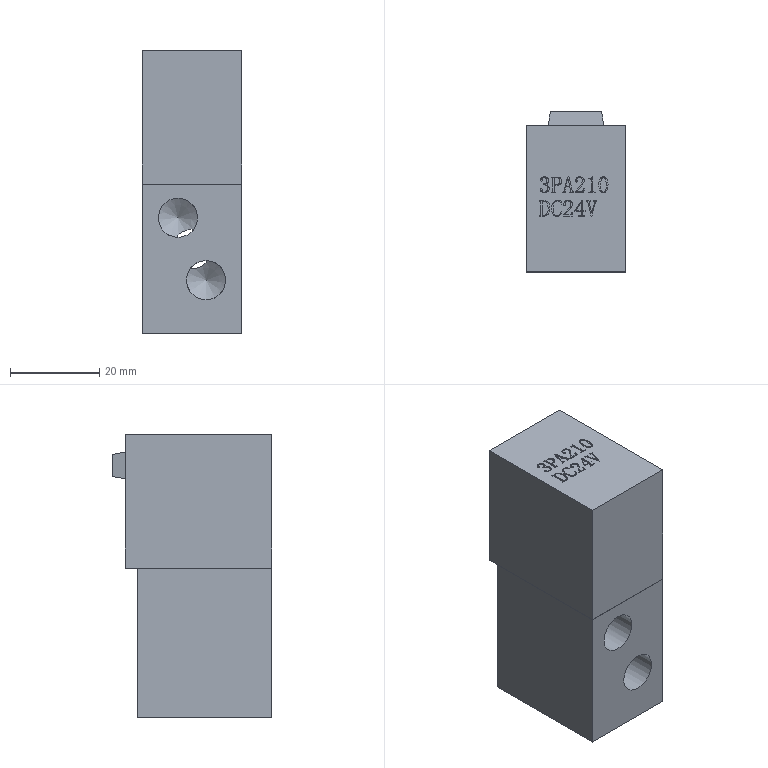Part | NX | 1 solid | 238 faces | box 22.3 x 35.8 x 63.52 mm | volume 40911 mm3 | plane 139 | spline 89 | cone 5 | cylinder 5 | commonest cylinder face diameters 8.8 x3 2.5 x2